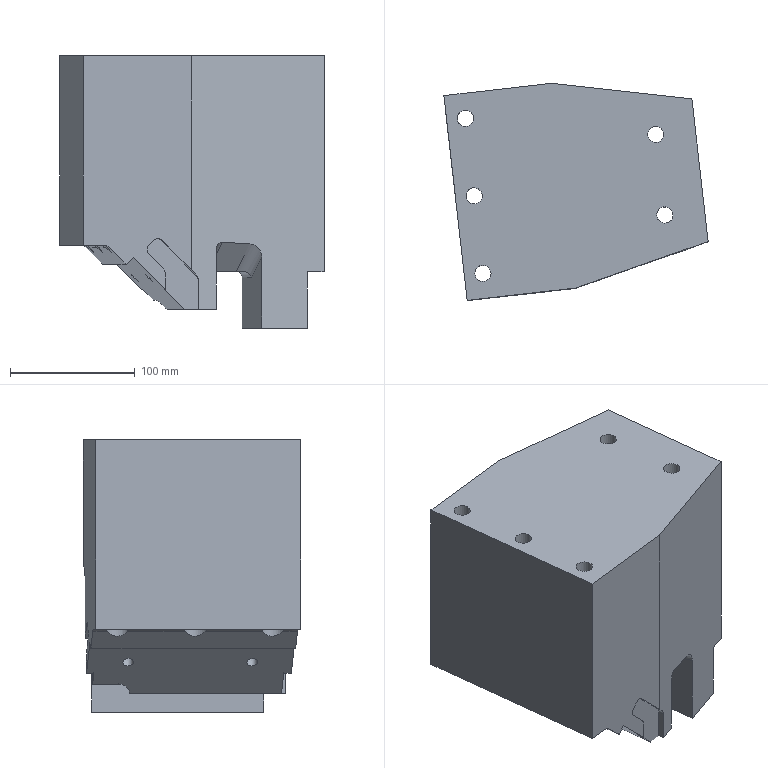Part | NX | features XQ 2 | 1 solid | 100 faces | box 211.582 x 173.788 x 218 mm | volume 5035756 mm3 | cylinder 44 | plane 41 | cone 8 | sphere 3 | spline 2 | torus 2 | commonest cylinder face diameters 20 x11 10 x9 12 x7 13 x5 5.2 x4 8 x4